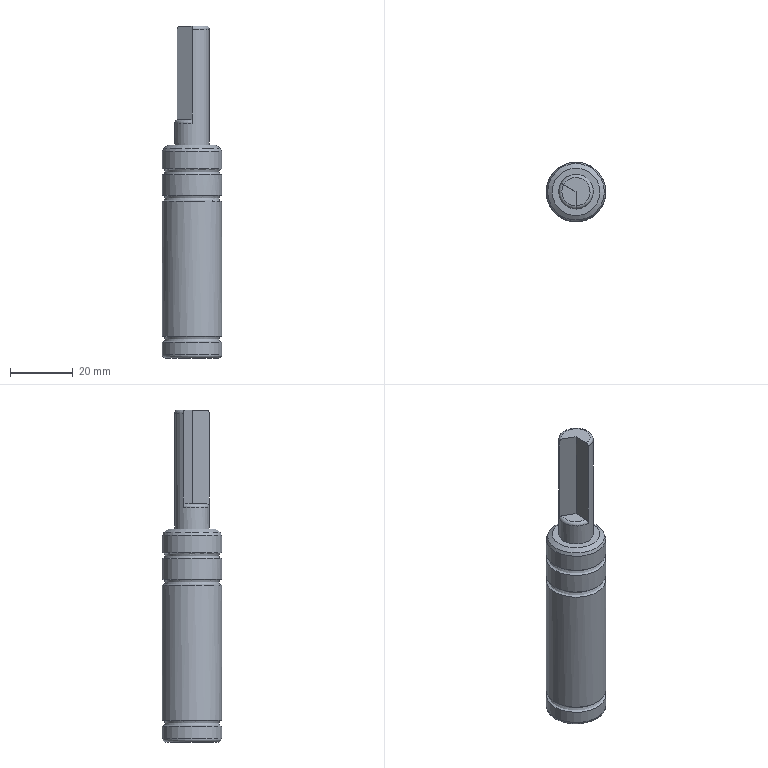Part | STEP file | GSV170-7_id502_x_t | 1 solid | 151 faces | box 19 x 19 x 106 mm | volume 21365 mm3 | other 73 | plane 59 | cylinder 9 | cone 4 | torus 3 | spline 3 | commonest cylinder face diameters 19 x6 5.1 x1 6 x1 11 x1